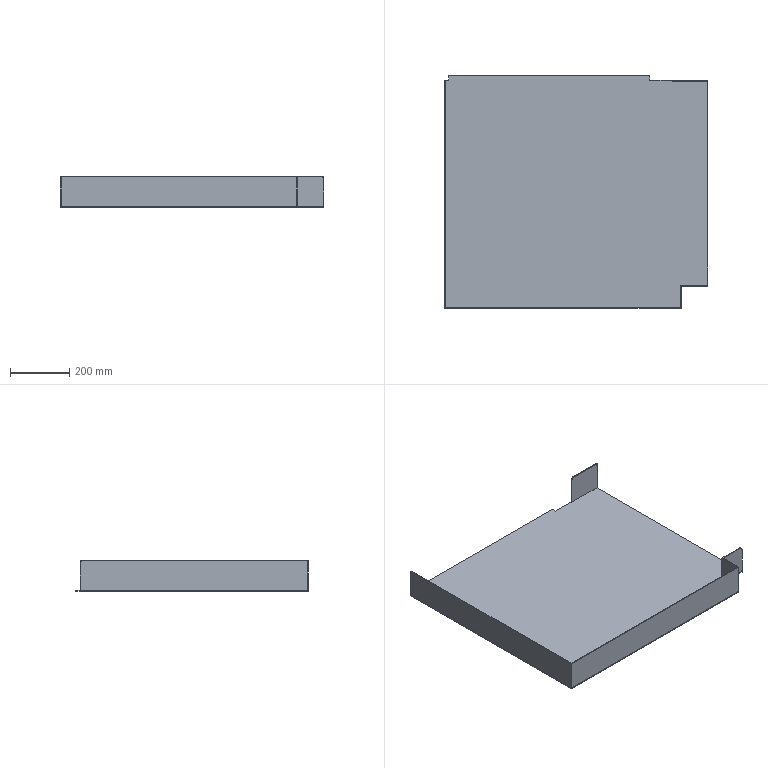Part | STEP file | PN_0049 checkered steel plate 1_Default<As Machined> | 3 solids | 33 faces | box 891 x 786 x 103 mm | volume 2627240 mm3 | plane 30 | cylinder 3 | commonest cylinder face diameters 20 x3